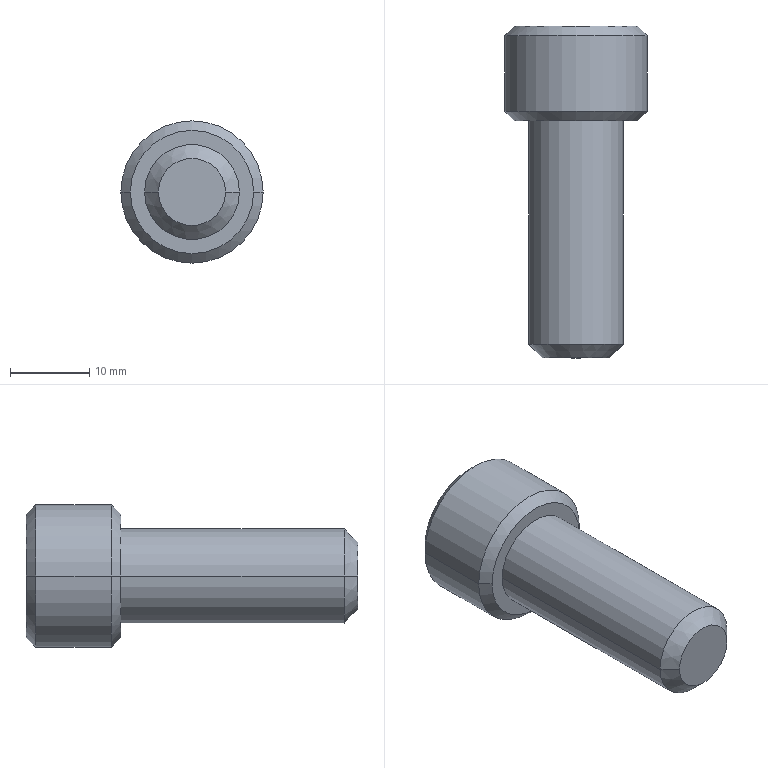Part | STEP file | BB62-M12-30L | 1 solid | 27 faces | box 18 x 42 x 18 mm | volume 5695 mm3 | plane 15 | cone 8 | cylinder 4 | commonest cylinder face diameters 12 x2 18 x2
STEP:
#1=CARTESIAN_POINT('',(0.,2.7,0.));
#2=VERTEX_POINT('',#1);
#3=CARTESIAN_POINT('',(5.715,6.,0.));
#4=VERTEX_POINT('',#3);
#5=CARTESIAN_POINT('',(0.,2.7,0.));
#6=DIRECTION('',(0.866,0.5,0.));
#7=VECTOR('',#6,1000.);
#8=LINE('',#5,#7);
#9=EDGE_CURVE('',#2,#4,#8,.T.);
#10=ORIENTED_EDGE('',*,*,#9,.F.);
#11=CARTESIAN_POINT('',(-5.715,6.,0.));
#12=VERTEX_POINT('',#11);
#13=CARTESIAN_POINT('',(0.,2.7,0.));
#14=DIRECTION('',(-0.866,0.5,0.));
#15=VECTOR('',#14,1000.);
#16=LINE('',#13,#15);
#17=EDGE_CURVE('',#2,#12,#16,.T.);
#18=ORIENTED_EDGE('',*,*,#17,.T.);
#19=CARTESIAN_POINT('',(-4.949,6.,2.857));
#20=VERTEX_POINT('',#19);
#21=CARTESIAN_POINT('',(0.,6.,0.));
#22=DIRECTION('',(0.,-1.,0.));
#23=DIRECTION('',(-1.,0.,0.));
#24=AXIS2_PLACEMENT_3D('',#21,#22,#23);
#25=CIRCLE('',#24,5.715);
#26=EDGE_CURVE('',#20,#12,#25,.T.);
#27=ORIENTED_EDGE('',*,*,#26,.F.);
#28=CARTESIAN_POINT('',(0.,6.,5.715));
#29=VERTEX_POINT('',#28);
#30=CARTESIAN_POINT('',(0.,6.,0.));
#31=DIRECTION('',(0.,-1.,0.));
#32=DIRECTION('',(-1.,0.,0.));
#33=AXIS2_PLACEMENT_3D('',#30,#31,#32);
#34=CIRCLE('',#33,5.715);
#35=EDGE_CURVE('',#29,#20,#34,.T.);
#36=ORIENTED_EDGE('',*,*,#35,.F.);
#37=CARTESIAN_POINT('',(4.949,6.,2.857));
#38=VERTEX_POINT('',#37);
#39=CARTESIAN_POINT('',(0.,6.,0.));
#40=DIRECTION('',(0.,-1.,0.));
#41=DIRECTION('',(-1.,0.,0.));
#42=AXIS2_PLACEMENT_3D('',#39,#40,#41);
#43=CIRCLE('',#42,5.715);
#44=EDGE_CURVE('',#38,#29,#43,.T.);
#45=ORIENTED_EDGE('',*,*,#44,.F.);
#46=CARTESIAN_POINT('',(0.,6.,0.));
#47=DIRECTION('',(0.,-1.,0.));
#48=DIRECTION('',(-1.,0.,0.));
#49=AXIS2_PLACEMENT_3D('',#46,#47,#48);
#50=CIRCLE('',#49,5.715);
#51=EDGE_CURVE('',#4,#38,#50,.T.);
#52=ORIENTED_EDGE('',*,*,#51,.F.);
#53=EDGE_LOOP('',(#10,#18,#27,#36,#45,#52));
#54=FACE_OUTER_BOUND('',#53,.T.);
#55=CARTESIAN_POINT('',(0.,1002.7,0.));
#56=DIRECTION('',(0.,1.,0.));
#57=DIRECTION('',(1.,0.,0.));
#58=AXIS2_PLACEMENT_3D('',#55,#56,#57);
#59=CONICAL_SURFACE('',#58,1732.051,1.047);
#60=ADVANCED_FACE('',(#54),#59,.F.);
#61=CARTESIAN_POINT('',(4.25,-30.,0.));
#62=VERTEX_POINT('',#61);
#63=CARTESIAN_POINT('',(-4.25,-30.,0.));
#64=VERTEX_POINT('',#63);
#65=CARTESIAN_POINT('',(0.,-30.,0.));
#66=DIRECTION('',(0.,1.,0.));
#67=DIRECTION('',(1.,0.,0.));
#68=AXIS2_PLACEMENT_3D('',#65,#66,#67);
#69=CIRCLE('',#68,4.25);
#70=EDGE_CURVE('',#62,#64,#69,.T.);
#71=ORIENTED_EDGE('',*,*,#70,.T.);
#72=CARTESIAN_POINT('',(-6.,-28.25,0.));
#73=VERTEX_POINT('',#72);
#74=CARTESIAN_POINT('',(-4.25,-30.,0.));
#75=DIRECTION('',(-0.7071,0.7071,0.));
#76=VECTOR('',#75,1000.);
#77=LINE('',#74,#76);
#78=EDGE_CURVE('',#64,#73,#77,.T.);
#79=ORIENTED_EDGE('',*,*,#78,.T.);
#80=CARTESIAN_POINT('',(6.,-28.25,0.));
#81=VERTEX_POINT('',#80);
#82=CARTESIAN_POINT('',(0.,-28.25,0.));
#83=DIRECTION('',(0.,-1.,0.));
#84=DIRECTION('',(-1.,0.,0.));
#85=AXIS2_PLACEMENT_3D('',#82,#83,#84);
#86=CIRCLE('',#85,6.);
#87=EDGE_CURVE('',#73,#81,#86,.T.);
#88=ORIENTED_EDGE('',*,*,#87,.T.);
#89=CARTESIAN_POINT('',(4.25,-30.,0.));
#90=DIRECTION('',(0.7071,0.7071,0.));
#91=VECTOR('',#90,1000.);
#92=LINE('',#89,#91);
#93=EDGE_CURVE('',#62,#81,#92,.T.);
#94=ORIENTED_EDGE('',*,*,#93,.F.);
#95=EDGE_LOOP('',(#71,#79,#88,#94));
#96=FACE_OUTER_BOUND('',#95,.T.);
#97=CARTESIAN_POINT('',(0.,-30.,0.));
#98=DIRECTION('',(0.,1.,0.));
#99=DIRECTION('',(1.,0.,0.));
#100=AXIS2_PLACEMENT_3D('',#97,#98,#99);
#101=CONICAL_SURFACE('',#100,4.25,0.7854);
#102=ADVANCED_FACE('',(#96),#101,.T.);
#103=ORIENTED_EDGE('',*,*,#87,.F.);
#104=CARTESIAN_POINT('',(-6.,0.,0.));
#105=VERTEX_POINT('',#104);
#106=CARTESIAN_POINT('',(-6.,-28.25,0.));
#107=DIRECTION('',(0.,1.,0.));
#108=VECTOR('',#107,1000.);
#109=LINE('',#106,#108);
#110=EDGE_CURVE('',#73,#105,#109,.T.);
#111=ORIENTED_EDGE('',*,*,#110,.T.);
#112=CARTESIAN_POINT('',(6.,0.,0.));
#113=VERTEX_POINT('',#112);
#114=CARTESIAN_POINT('',(0.,0.,0.));
#115=DIRECTION('',(0.,-1.,0.));
#116=DIRECTION('',(-1.,0.,0.));
#117=AXIS2_PLACEMENT_3D('',#114,#115,#116);
#118=CIRCLE('',#117,6.);
#119=EDGE_CURVE('',#105,#113,#118,.T.);
#120=ORIENTED_EDGE('',*,*,#119,.T.);
#121=CARTESIAN_POINT('',(6.,-28.25,0.));
#122=DIRECTION('',(0.,1.,0.));
#123=VECTOR('',#122,1000.);
#124=LINE('',#121,#123);
#125=EDGE_CURVE('',#81,#113,#124,.T.);
#126=ORIENTED_EDGE('',*,*,#125,.F.);
#127=EDGE_LOOP('',(#103,#111,#120,#126));
#128=FACE_OUTER_BOUND('',#127,.T.);
#129=CARTESIAN_POINT('',(0.,-28.25,0.));
#130=DIRECTION('',(0.,1.,0.));
#131=DIRECTION('',(1.,0.,0.));
#132=AXIS2_PLACEMENT_3D('',#129,#130,#131);
#133=CYLINDRICAL_SURFACE('',#132,6.);
#134=ADVANCED_FACE('',(#128),#133,.T.);
#135=CARTESIAN_POINT('',(-7.8,12.,0.));
#136=VERTEX_POINT('',#135);
#137=CARTESIAN_POINT('',(7.8,12.,0.));
#138=VERTEX_POINT('',#137);
#139=CARTESIAN_POINT('',(0.,12.,0.));
#140=DIRECTION('',(0.,-1.,0.));
#141=DIRECTION('',(-1.,0.,0.));
#142=AXIS2_PLACEMENT_3D('',#139,#140,#141);
#143=CIRCLE('',#142,7.8);
#144=EDGE_CURVE('',#136,#138,#143,.T.);
#145=ORIENTED_EDGE('',*,*,#144,.T.);
#146=CARTESIAN_POINT('',(9.,10.8,0.));
#147=VERTEX_POINT('',#146);
#148=CARTESIAN_POINT('',(9.,10.8,0.));
#149=DIRECTION('',(0.7071,-0.7071,0.));
#150=VECTOR('',#149,1000.);
#151=LINE('',#148,#150);
#152=EDGE_CURVE('',#138,#147,#151,.T.);
#153=ORIENTED_EDGE('',*,*,#152,.T.);
#154=CARTESIAN_POINT('',(-9.,10.8,0.));
#155=VERTEX_POINT('',#154);
#156=CARTESIAN_POINT('',(0.,10.8,0.));
#157=DIRECTION('',(0.,-1.,0.));
#158=DIRECTION('',(-1.,0.,0.));
#159=AXIS2_PLACEMENT_3D('',#156,#157,#158);
#160=CIRCLE('',#159,9.);
#161=EDGE_CURVE('',#155,#147,#160,.T.);
#162=ORIENTED_EDGE('',*,*,#161,.F.);
#163=CARTESIAN_POINT('',(-9.,10.8,0.));
#164=DIRECTION('',(-0.7071,-0.7071,0.));
#165=VECTOR('',#164,1000.);
#166=LINE('',#163,#165);
#167=EDGE_CURVE('',#136,#155,#166,.T.);
#168=ORIENTED_EDGE('',*,*,#167,.F.);
#169=EDGE_LOOP('',(#145,#153,#162,#168));
#170=FACE_OUTER_BOUND('',#169,.T.);
#171=CARTESIAN_POINT('',(0.,10.8,0.));
#172=DIRECTION('',(0.,-1.,0.));
#173=DIRECTION('',(-1.,0.,0.));
#174=AXIS2_PLACEMENT_3D('',#171,#172,#173);
#175=CONICAL_SURFACE('',#174,9.,0.7854);
#176=ADVANCED_FACE('',(#170),#175,.T.);
#177=ORIENTED_EDGE('',*,*,#161,.T.);
#178=CARTESIAN_POINT('',(9.,1.2,0.));
#179=VERTEX_POINT('',#178);
#180=CARTESIAN_POINT('',(9.,1.62,0.));
#181=DIRECTION('',(0.,-1.,0.));
#182=VECTOR('',#181,1000.);
#183=LINE('',#180,#182);
#184=EDGE_CURVE('',#147,#179,#183,.T.);
#185=ORIENTED_EDGE('',*,*,#184,.T.);
#186=CARTESIAN_POINT('',(-9.,1.2,0.));
#187=VERTEX_POINT('',#186);
#188=CARTESIAN_POINT('',(0.,1.2,0.));
#189=DIRECTION('',(0.,-1.,0.));
#190=DIRECTION('',(-1.,0.,0.));
#191=AXIS2_PLACEMENT_3D('',#188,#189,#190);
#192=CIRCLE('',#191,9.);
#193=EDGE_CURVE('',#187,#179,#192,.T.);
#194=ORIENTED_EDGE('',*,*,#193,.F.);
#195=CARTESIAN_POINT('',(-9.,1.62,0.));
#196=DIRECTION('',(0.,-1.,0.));
#197=VECTOR('',#196,1000.);
#198=LINE('',#195,#197);
#199=EDGE_CURVE('',#155,#187,#198,.T.);
#200=ORIENTED_EDGE('',*,*,#199,.F.);
#201=EDGE_LOOP('',(#177,#185,#194,#200));
#202=FACE_OUTER_BOUND('',#201,.T.);
#203=CARTESIAN_POINT('',(0.,1.62,0.));
#204=DIRECTION('',(0.,-1.,0.));
#205=DIRECTION('',(-1.,0.,0.));
#206=AXIS2_PLACEMENT_3D('',#203,#204,#205);
#207=CYLINDRICAL_SURFACE('',#206,9.);
#208=ADVANCED_FACE('',(#202),#207,.T.);
#209=CARTESIAN_POINT('',(-7.8,0.,0.));
#210=VERTEX_POINT('',#209);
#211=CARTESIAN_POINT('',(7.8,0.,0.));
#212=VERTEX_POINT('',#211);
#213=CARTESIAN_POINT('',(0.,0.,0.));
#214=DIRECTION('',(0.,-1.,0.));
#215=DIRECTION('',(-1.,0.,0.));
#216=AXIS2_PLACEMENT_3D('',#213,#214,#215);
#217=CIRCLE('',#216,7.8);
#218=EDGE_CURVE('',#210,#212,#217,.T.);
#219=ORIENTED_EDGE('',*,*,#218,.F.);
#220=CARTESIAN_POINT('',(-7.8,0.,0.));
#221=DIRECTION('',(-0.7071,0.7071,0.));
#222=VECTOR('',#221,1000.);
#223=LINE('',#220,#222);
#224=EDGE_CURVE('',#210,#187,#223,.T.);
#225=ORIENTED_EDGE('',*,*,#224,.T.);
#226=ORIENTED_EDGE('',*,*,#193,.T.);
#227=CARTESIAN_POINT('',(7.8,0.,0.));
#228=DIRECTION('',(0.7071,0.7071,0.));
#229=VECTOR('',#228,1000.);
#230=LINE('',#227,#229);
#231=EDGE_CURVE('',#212,#179,#230,.T.);
#232=ORIENTED_EDGE('',*,*,#231,.F.);
#233=EDGE_LOOP('',(#219,#225,#226,#232));
#234=FACE_OUTER_BOUND('',#233,.T.);
#235=CARTESIAN_POINT('',(0.,0.,0.));
#236=DIRECTION('',(0.,1.,0.));
#237=DIRECTION('',(1.,0.,0.));
#238=AXIS2_PLACEMENT_3D('',#235,#236,#237);
#239=CONICAL_SURFACE('',#238,7.8,0.7854);
#240=ADVANCED_FACE('',(#234),#239,.T.);
#241=ORIENTED_EDGE('',*,*,#144,.F.);
#242=CARTESIAN_POINT('',(0.,12.,0.));
#243=DIRECTION('',(0.,-1.,0.));
#244=DIRECTION('',(-1.,0.,0.));
#245=AXIS2_PLACEMENT_3D('',#242,#243,#244);
#246=CIRCLE('',#245,7.8);
#247=EDGE_CURVE('',#138,#136,#246,.T.);
#248=ORIENTED_EDGE('',*,*,#247,.F.);
#249=EDGE_LOOP('',(#241,#248));
#250=FACE_OUTER_BOUND('',#249,.T.);
#251=CARTESIAN_POINT('',(0.,12.,-5.715));
#252=VERTEX_POINT('',#251);
#253=CARTESIAN_POINT('',(-4.949,12.,-2.857));
#254=VERTEX_POINT('',#253);
#255=CARTESIAN_POINT('',(0.,12.,-5.715));
#256=DIRECTION('',(-0.866,0.,0.5));
#257=VECTOR('',#256,1000.);
#258=LINE('',#255,#257);
#259=EDGE_CURVE('',#252,#254,#258,.T.);
#260=ORIENTED_EDGE('',*,*,#259,.F.);
#261=CARTESIAN_POINT('',(4.949,12.,-2.857));
#262=VERTEX_POINT('',#261);
#263=CARTESIAN_POINT('',(4.949,12.,-2.857));
#264=DIRECTION('',(-0.866,0.,-0.5));
#265=VECTOR('',#264,1000.);
#266=LINE('',#263,#265);
#267=EDGE_CURVE('',#262,#252,#266,.T.);
#268=ORIENTED_EDGE('',*,*,#267,.F.);
#269=CARTESIAN_POINT('',(4.949,12.,2.857));
#270=VERTEX_POINT('',#269);
#271=CARTESIAN_POINT('',(4.949,12.,2.857));
#272=DIRECTION('',(0.,0.,-1.));
#273=VECTOR('',#272,1000.);
#274=LINE('',#271,#273);
#275=EDGE_CURVE('',#270,#262,#274,.T.);
#276=ORIENTED_EDGE('',*,*,#275,.F.);
#277=CARTESIAN_POINT('',(0.,12.,5.715));
#278=VERTEX_POINT('',#277);
#279=CARTESIAN_POINT('',(0.,12.,5.715));
#280=DIRECTION('',(0.866,0.,-0.5));
#281=VECTOR('',#280,1000.);
#282=LINE('',#279,#281);
#283=EDGE_CURVE('',#278,#270,#282,.T.);
#284=ORIENTED_EDGE('',*,*,#283,.F.);
#285=CARTESIAN_POINT('',(-4.949,12.,2.857));
#286=VERTEX_POINT('',#285);
#287=CARTESIAN_POINT('',(-4.949,12.,2.857));
#288=DIRECTION('',(0.866,0.,0.5));
#289=VECTOR('',#288,1000.);
#290=LINE('',#287,#289);
#291=EDGE_CURVE('',#286,#278,#290,.T.);
#292=ORIENTED_EDGE('',*,*,#291,.F.);
#293=CARTESIAN_POINT('',(-4.949,12.,-2.857));
#294=DIRECTION('',(0.,0.,1.));
#295=VECTOR('',#294,1000.);
#296=LINE('',#293,#295);
#297=EDGE_CURVE('',#254,#286,#296,.T.);
#298=ORIENTED_EDGE('',*,*,#297,.F.);
#299=EDGE_LOOP('',(#260,#268,#276,#284,#292,#298));
#300=FACE_BOUND('',#299,.T.);
#301=CARTESIAN_POINT('',(7.8,12.,0.));
#302=DIRECTION('',(0.,1.,0.));
#303=DIRECTION('',(1.,0.,0.));
#304=AXIS2_PLACEMENT_3D('',#301,#302,#303);
#305=PLANE('',#304);
#306=ADVANCED_FACE('',(#250,#300),#305,.T.);
#307=CARTESIAN_POINT('',(0.,0.,0.));
#308=DIRECTION('',(0.,-1.,0.));
#309=DIRECTION('',(-1.,0.,0.));
#310=AXIS2_PLACEMENT_3D('',#307,#308,#309);
#311=CIRCLE('',#310,6.);
#312=EDGE_CURVE('',#113,#105,#311,.T.);
#313=ORIENTED_EDGE('',*,*,#312,.F.);
#314=ORIENTED_EDGE('',*,*,#119,.F.);
#315=EDGE_LOOP('',(#313,#314));
#316=FACE_BOUND('',#315,.T.);
#317=CARTESIAN_POINT('',(0.,0.,0.));
#318=DIRECTION('',(0.,-1.,0.));
#319=DIRECTION('',(-1.,0.,0.));
#320=AXIS2_PLACEMENT_3D('',#317,#318,#319);
#321=CIRCLE('',#320,7.8);
#322=EDGE_CURVE('',#212,#210,#321,.T.);
#323=ORIENTED_EDGE('',*,*,#322,.T.);
#324=ORIENTED_EDGE('',*,*,#218,.T.);
#325=EDGE_LOOP('',(#323,#324));
#326=FACE_OUTER_BOUND('',#325,.T.);
#327=CARTESIAN_POINT('',(0.,0.,0.));
#328=DIRECTION('',(0.,-1.,0.));
#329=DIRECTION('',(-1.,0.,0.));
#330=AXIS2_PLACEMENT_3D('',#327,#328,#329);
#331=PLANE('',#330);
#332=ADVANCED_FACE('',(#316,#326),#331,.T.);
#333=ORIENTED_EDGE('',*,*,#224,.F.);
#334=ORIENTED_EDGE('',*,*,#322,.F.);
#335=ORIENTED_EDGE('',*,*,#231,.T.);
#336=CARTESIAN_POINT('',(0.,1.2,0.));
#337=DIRECTION('',(0.,-1.,0.));
#338=DIRECTION('',(-1.,0.,0.));
#339=AXIS2_PLACEMENT_3D('',#336,#337,#338);
#340=CIRCLE('',#339,9.);
#341=EDGE_CURVE('',#179,#187,#340,.T.);
#342=ORIENTED_EDGE('',*,*,#341,.T.);
#343=EDGE_LOOP('',(#333,#334,#335,#342));
#344=FACE_OUTER_BOUND('',#343,.T.);
#345=CARTESIAN_POINT('',(0.,0.,0.));
#346=DIRECTION('',(0.,1.,0.));
#347=DIRECTION('',(1.,0.,0.));
#348=AXIS2_PLACEMENT_3D('',#345,#346,#347);
#349=CONICAL_SURFACE('',#348,7.8,0.7854);
#350=ADVANCED_FACE('',(#344),#349,.T.);
#351=ORIENTED_EDGE('',*,*,#184,.F.);
#352=CARTESIAN_POINT('',(0.,10.8,0.));
#353=DIRECTION('',(0.,-1.,0.));
#354=DIRECTION('',(-1.,0.,0.));
#355=AXIS2_PLACEMENT_3D('',#352,#353,#354);
#356=CIRCLE('',#355,9.);
#357=EDGE_CURVE('',#147,#155,#356,.T.);
#358=ORIENTED_EDGE('',*,*,#357,.T.);
#359=ORIENTED_EDGE('',*,*,#199,.T.);
#360=ORIENTED_EDGE('',*,*,#341,.F.);
#361=EDGE_LOOP('',(#351,#358,#359,#360));
#362=FACE_OUTER_BOUND('',#361,.T.);
#363=CARTESIAN_POINT('',(0.,1.62,0.));
#364=DIRECTION('',(0.,-1.,0.));
#365=DIRECTION('',(-1.,0.,0.));
#366=AXIS2_PLACEMENT_3D('',#363,#364,#365);
#367=CYLINDRICAL_SURFACE('',#366,9.);
#368=ADVANCED_FACE('',(#362),#367,.T.);
#369=ORIENTED_EDGE('',*,*,#152,.F.);
#370=ORIENTED_EDGE('',*,*,#247,.T.);
#371=ORIENTED_EDGE('',*,*,#167,.T.);
#372=ORIENTED_EDGE('',*,*,#357,.F.);
#373=EDGE_LOOP('',(#369,#370,#371,#372));
#374=FACE_OUTER_BOUND('',#373,.T.);
#375=CARTESIAN_POINT('',(0.,10.8,0.));
#376=DIRECTION('',(0.,-1.,0.));
#377=DIRECTION('',(-1.,0.,0.));
#378=AXIS2_PLACEMENT_3D('',#375,#376,#377);
#379=CONICAL_SURFACE('',#378,9.,0.7854);
#380=ADVANCED_FACE('',(#374),#379,.T.);
#381=ORIENTED_EDGE('',*,*,#110,.F.);
#382=CARTESIAN_POINT('',(0.,-28.25,0.));
#383=DIRECTION('',(0.,-1.,0.));
#384=DIRECTION('',(-1.,0.,0.));
#385=AXIS2_PLACEMENT_3D('',#382,#383,#384);
#386=CIRCLE('',#385,6.);
#387=EDGE_CURVE('',#81,#73,#386,.T.);
#388=ORIENTED_EDGE('',*,*,#387,.F.);
#389=ORIENTED_EDGE('',*,*,#125,.T.);
#390=ORIENTED_EDGE('',*,*,#312,.T.);
#391=EDGE_LOOP('',(#381,#388,#389,#390));
#392=FACE_OUTER_BOUND('',#391,.T.);
#393=CARTESIAN_POINT('',(0.,-28.25,0.));
#394=DIRECTION('',(0.,1.,0.));
#395=DIRECTION('',(1.,0.,0.));
#396=AXIS2_PLACEMENT_3D('',#393,#394,#395);
#397=CYLINDRICAL_SURFACE('',#396,6.);
#398=ADVANCED_FACE('',(#392),#397,.T.);
#399=ORIENTED_EDGE('',*,*,#70,.F.);
#400=CARTESIAN_POINT('',(0.,-30.,0.));
#401=DIRECTION('',(0.,1.,0.));
#402=DIRECTION('',(1.,0.,0.));
#403=AXIS2_PLACEMENT_3D('',#400,#401,#402);
#404=CIRCLE('',#403,4.25);
#405=EDGE_CURVE('',#64,#62,#404,.T.);
#406=ORIENTED_EDGE('',*,*,#405,.F.);
#407=EDGE_LOOP('',(#399,#406));
#408=FACE_OUTER_BOUND('',#407,.T.);
#409=CARTESIAN_POINT('',(0.,-30.,0.));
#410=DIRECTION('',(0.,-1.,0.));
#411=DIRECTION('',(-1.,0.,0.));
#412=AXIS2_PLACEMENT_3D('',#409,#410,#411);
#413=PLANE('',#412);
#414=ADVANCED_FACE('',(#408),#413,.T.);
#415=ORIENTED_EDGE('',*,*,#78,.F.);
#416=ORIENTED_EDGE('',*,*,#405,.T.);
#417=ORIENTED_EDGE('',*,*,#93,.T.);
#418=ORIENTED_EDGE('',*,*,#387,.T.);
#419=EDGE_LOOP('',(#415,#416,#417,#418));
#420=FACE_OUTER_BOUND('',#419,.T.);
#421=CARTESIAN_POINT('',(0.,-30.,0.));
#422=DIRECTION('',(0.,1.,0.));
#423=DIRECTION('',(1.,0.,0.));
#424=AXIS2_PLACEMENT_3D('',#421,#422,#423);
#425=CONICAL_SURFACE('',#424,4.25,0.7854);
#426=ADVANCED_FACE('',(#420),#425,.T.);
#427=CARTESIAN_POINT('',(4.949,6.,-2.858));
#428=VERTEX_POINT('',#427);
#429=CARTESIAN_POINT('',(0.,6.,-5.715));
#430=VERTEX_POINT('',#429);
#431=CARTESIAN_POINT('',(4.949,6.,-2.857));
#432=DIRECTION('',(-0.866,0.,-0.5));
#433=VECTOR('',#432,1000.);
#434=LINE('',#431,#433);
#435=EDGE_CURVE('',#428,#430,#434,.T.);
#436=ORIENTED_EDGE('',*,*,#435,.F.);
#437=CARTESIAN_POINT('',(4.949,12.,-2.857));
#438=DIRECTION('',(0.,-1.,0.));
#439=VECTOR('',#438,1000.);
#440=LINE('',#437,#439);
#441=EDGE_CURVE('',#262,#428,#440,.T.);
#442=ORIENTED_EDGE('',*,*,#441,.F.);
#443=ORIENTED_EDGE('',*,*,#267,.T.);
#444=CARTESIAN_POINT('',(0.,12.,-5.715));
#445=DIRECTION('',(0.,-1.,0.));
#446=VECTOR('',#445,1000.);
#447=LINE('',#444,#446);
#448=EDGE_CURVE('',#252,#430,#447,.T.);
#449=ORIENTED_EDGE('',*,*,#448,.T.);
#450=EDGE_LOOP('',(#436,#442,#443,#449));
#451=FACE_OUTER_BOUND('',#450,.T.);
#452=CARTESIAN_POINT('',(4.949,12.,-2.857));
#453=DIRECTION('',(-0.5,0.,0.866));
#454=DIRECTION('',(0.866,0.,0.5));
#455=AXIS2_PLACEMENT_3D('',#452,#453,#454);
#456=PLANE('',#455);
#457=ADVANCED_FACE('',(#451),#456,.T.);
#458=CARTESIAN_POINT('',(-4.949,6.,-2.857));
#459=VERTEX_POINT('',#458);
#460=CARTESIAN_POINT('',(0.,6.,-5.715));
#461=DIRECTION('',(-0.866,0.,0.5));
#462=VECTOR('',#461,1000.);
#463=LINE('',#460,#462);
#464=EDGE_CURVE('',#430,#459,#463,.T.);
#465=ORIENTED_EDGE('',*,*,#464,.F.);
#466=ORIENTED_EDGE('',*,*,#448,.F.);
#467=ORIENTED_EDGE('',*,*,#259,.T.);
#468=CARTESIAN_POINT('',(-4.949,12.,-2.857));
#469=DIRECTION('',(0.,-1.,0.));
#470=VECTOR('',#469,1000.);
#471=LINE('',#468,#470);
#472=EDGE_CURVE('',#254,#459,#471,.T.);
#473=ORIENTED_EDGE('',*,*,#472,.T.);
#474=EDGE_LOOP('',(#465,#466,#467,#473));
#475=FACE_OUTER_BOUND('',#474,.T.);
#476=CARTESIAN_POINT('',(0.,12.,-5.715));
#477=DIRECTION('',(0.5,0.,0.866));
#478=DIRECTION('',(0.866,0.,-0.5));
#479=AXIS2_PLACEMENT_3D('',#476,#477,#478);
#480=PLANE('',#479);
#481=ADVANCED_FACE('',(#475),#480,.T.);
#482=CARTESIAN_POINT('',(-4.949,6.,-2.857));
#483=DIRECTION('',(0.,0.,1.));
#484=VECTOR('',#483,1000.);
#485=LINE('',#482,#484);
#486=EDGE_CURVE('',#459,#20,#485,.T.);
#487=ORIENTED_EDGE('',*,*,#486,.F.);
#488=ORIENTED_EDGE('',*,*,#472,.F.);
#489=ORIENTED_EDGE('',*,*,#297,.T.);
#490=CARTESIAN_POINT('',(-4.949,12.,2.857));
#491=DIRECTION('',(0.,-1.,0.));
#492=VECTOR('',#491,1000.);
#493=LINE('',#490,#492);
#494=EDGE_CURVE('',#286,#20,#493,.T.);
#495=ORIENTED_EDGE('',*,*,#494,.T.);
#496=EDGE_LOOP('',(#487,#488,#489,#495));
#497=FACE_OUTER_BOUND('',#496,.T.);
#498=CARTESIAN_POINT('',(-4.949,12.,-2.857));
#499=DIRECTION('',(1.,0.,0.));
#500=DIRECTION('',(0.,0.,-1.));
#501=AXIS2_PLACEMENT_3D('',#498,#499,#500);
#502=PLANE('',#501);
#503=ADVANCED_FACE('',(#497),#502,.T.);
#504=CARTESIAN_POINT('',(-4.949,6.,2.857));
#505=DIRECTION('',(0.866,0.,0.5));
#506=VECTOR('',#505,1000.);
#507=LINE('',#504,#506);
#508=EDGE_CURVE('',#20,#29,#507,.T.);
#509=ORIENTED_EDGE('',*,*,#508,.F.);
#510=ORIENTED_EDGE('',*,*,#494,.F.);
#511=ORIENTED_EDGE('',*,*,#291,.T.);
#512=CARTESIAN_POINT('',(0.,12.,5.715));
#513=DIRECTION('',(0.,-1.,0.));
#514=VECTOR('',#513,1000.);
#515=LINE('',#512,#514);
#516=EDGE_CURVE('',#278,#29,#515,.T.);
#517=ORIENTED_EDGE('',*,*,#516,.T.);
#518=EDGE_LOOP('',(#509,#510,#511,#517));
#519=FACE_OUTER_BOUND('',#518,.T.);
#520=CARTESIAN_POINT('',(-4.949,12.,2.857));
#521=DIRECTION('',(0.5,0.,-0.866));
#522=DIRECTION('',(-0.866,0.,-0.5));
#523=AXIS2_PLACEMENT_3D('',#520,#521,#522);
#524=PLANE('',#523);
#525=ADVANCED_FACE('',(#519),#524,.T.);
#526=CARTESIAN_POINT('',(0.,6.,5.715));
#527=DIRECTION('',(0.866,0.,-0.5));
#528=VECTOR('',#527,1000.);
#529=LINE('',#526,#528);
#530=EDGE_CURVE('',#29,#38,#529,.T.);
#531=ORIENTED_EDGE('',*,*,#530,.F.);
#532=ORIENTED_EDGE('',*,*,#516,.F.);
#533=ORIENTED_EDGE('',*,*,#283,.T.);
#534=CARTESIAN_POINT('',(4.949,12.,2.857));
#535=DIRECTION('',(0.,-1.,0.));
#536=VECTOR('',#535,1000.);
#537=LINE('',#534,#536);
#538=EDGE_CURVE('',#270,#38,#537,.T.);
#539=ORIENTED_EDGE('',*,*,#538,.T.);
#540=EDGE_LOOP('',(#531,#532,#533,#539));
#541=FACE_OUTER_BOUND('',#540,.T.);
#542=CARTESIAN_POINT('',(0.,12.,5.715));
#543=DIRECTION('',(-0.5,0.,-0.866));
#544=DIRECTION('',(-0.866,0.,0.5));
#545=AXIS2_PLACEMENT_3D('',#542,#543,#544);
#546=PLANE('',#545);
#547=ADVANCED_FACE('',(#541),#546,.T.);
#548=CARTESIAN_POINT('',(4.949,6.,2.857));
#549=DIRECTION('',(0.,0.,-1.));
#550=VECTOR('',#549,1000.);
#551=LINE('',#548,#550);
#552=EDGE_CURVE('',#38,#428,#551,.T.);
#553=ORIENTED_EDGE('',*,*,#552,.F.);
#554=ORIENTED_EDGE('',*,*,#538,.F.);
#555=ORIENTED_EDGE('',*,*,#275,.T.);
#556=ORIENTED_EDGE('',*,*,#441,.T.);
#557=EDGE_LOOP('',(#553,#554,#555,#556));
#558=FACE_OUTER_BOUND('',#557,.T.);
#559=CARTESIAN_POINT('',(4.949,12.,2.857));
#560=DIRECTION('',(-1.,0.,0.));
#561=DIRECTION('',(0.,0.,1.));
#562=AXIS2_PLACEMENT_3D('',#559,#560,#561);
#563=PLANE('',#562);
#564=ADVANCED_FACE('',(#558),#563,.T.);
#565=ORIENTED_EDGE('',*,*,#435,.T.);
#566=CARTESIAN_POINT('',(0.,6.,0.));
#567=DIRECTION('',(0.,-1.,0.));
#568=DIRECTION('',(-1.,0.,0.));
#569=AXIS2_PLACEMENT_3D('',#566,#567,#568);
#570=CIRCLE('',#569,5.715);
#571=EDGE_CURVE('',#430,#428,#570,.T.);
#572=ORIENTED_EDGE('',*,*,#571,.T.);
#573=EDGE_LOOP('',(#565,#572));
#574=FACE_OUTER_BOUND('',#573,.T.);
#575=CARTESIAN_POINT('',(0.,6.,0.));
#576=DIRECTION('',(0.,1.,0.));
#577=DIRECTION('',(1.,0.,0.));
#578=AXIS2_PLACEMENT_3D('',#575,#576,#577);
#579=PLANE('',#578);
#580=ADVANCED_FACE('',(#574),#579,.F.);
#581=ORIENTED_EDGE('',*,*,#552,.T.);
#582=CARTESIAN_POINT('',(0.,6.,0.));
#583=DIRECTION('',(0.,-1.,0.));
#584=DIRECTION('',(-1.,0.,0.));
#585=AXIS2_PLACEMENT_3D('',#582,#583,#584);
#586=CIRCLE('',#585,5.715);
#587=EDGE_CURVE('',#428,#4,#586,.T.);
#588=ORIENTED_EDGE('',*,*,#587,.T.);
#589=ORIENTED_EDGE('',*,*,#51,.T.);
#590=EDGE_LOOP('',(#581,#588,#589));
#591=FACE_OUTER_BOUND('',#590,.T.);
#592=CARTESIAN_POINT('',(0.,6.,0.));
#593=DIRECTION('',(0.,1.,0.));
#594=DIRECTION('',(1.,0.,0.));
#595=AXIS2_PLACEMENT_3D('',#592,#593,#594);
#596=PLANE('',#595);
#597=ADVANCED_FACE('',(#591),#596,.F.);
#598=ORIENTED_EDGE('',*,*,#530,.T.);
#599=ORIENTED_EDGE('',*,*,#44,.T.);
#600=EDGE_LOOP('',(#598,#599));
#601=FACE_OUTER_BOUND('',#600,.T.);
#602=CARTESIAN_POINT('',(0.,6.,0.));
#603=DIRECTION('',(0.,1.,0.));
#604=DIRECTION('',(1.,0.,0.));
#605=AXIS2_PLACEMENT_3D('',#602,#603,#604);
#606=PLANE('',#605);
#607=ADVANCED_FACE('',(#601),#606,.F.);
#608=ORIENTED_EDGE('',*,*,#508,.T.);
#609=ORIENTED_EDGE('',*,*,#35,.T.);
#610=EDGE_LOOP('',(#608,#609));
#611=FACE_OUTER_BOUND('',#610,.T.);
#612=CARTESIAN_POINT('',(0.,6.,0.));
#613=DIRECTION('',(0.,1.,0.));
#614=DIRECTION('',(1.,0.,0.));
#615=AXIS2_PLACEMENT_3D('',#612,#613,#614);
#616=PLANE('',#615);
#617=ADVANCED_FACE('',(#611),#616,.F.);
#618=ORIENTED_EDGE('',*,*,#486,.T.);
#619=ORIENTED_EDGE('',*,*,#26,.T.);
#620=CARTESIAN_POINT('',(0.,6.,0.));
#621=DIRECTION('',(0.,-1.,0.));
#622=DIRECTION('',(-1.,0.,0.));
#623=AXIS2_PLACEMENT_3D('',#620,#621,#622);
#624=CIRCLE('',#623,5.715);
#625=EDGE_CURVE('',#12,#459,#624,.T.);
#626=ORIENTED_EDGE('',*,*,#625,.T.);
#627=EDGE_LOOP('',(#618,#619,#626));
#628=FACE_OUTER_BOUND('',#627,.T.);
#629=CARTESIAN_POINT('',(0.,6.,0.));
#630=DIRECTION('',(0.,1.,0.));
#631=DIRECTION('',(1.,0.,0.));
#632=AXIS2_PLACEMENT_3D('',#629,#630,#631);
#633=PLANE('',#632);
#634=ADVANCED_FACE('',(#628),#633,.F.);
#635=ORIENTED_EDGE('',*,*,#464,.T.);
#636=CARTESIAN_POINT('',(0.,6.,0.));
#637=DIRECTION('',(0.,-1.,0.));
#638=DIRECTION('',(-1.,0.,0.));
#639=AXIS2_PLACEMENT_3D('',#636,#637,#638);
#640=CIRCLE('',#639,5.715);
#641=EDGE_CURVE('',#459,#430,#640,.T.);
#642=ORIENTED_EDGE('',*,*,#641,.T.);
#643=EDGE_LOOP('',(#635,#642));
#644=FACE_OUTER_BOUND('',#643,.T.);
#645=CARTESIAN_POINT('',(0.,6.,0.));
#646=DIRECTION('',(0.,1.,0.));
#647=DIRECTION('',(1.,0.,0.));
#648=AXIS2_PLACEMENT_3D('',#645,#646,#647);
#649=PLANE('',#648);
#650=ADVANCED_FACE('',(#644),#649,.F.);
#651=ORIENTED_EDGE('',*,*,#17,.F.);
#652=ORIENTED_EDGE('',*,*,#9,.T.);
#653=ORIENTED_EDGE('',*,*,#587,.F.);
#654=ORIENTED_EDGE('',*,*,#571,.F.);
#655=ORIENTED_EDGE('',*,*,#641,.F.);
#656=ORIENTED_EDGE('',*,*,#625,.F.);
#657=EDGE_LOOP('',(#651,#652,#653,#654,#655,#656));
#658=FACE_OUTER_BOUND('',#657,.T.);
#659=CARTESIAN_POINT('',(0.,1002.7,0.));
#660=DIRECTION('',(0.,1.,0.));
#661=DIRECTION('',(1.,0.,0.));
#662=AXIS2_PLACEMENT_3D('',#659,#660,#661);
#663=CONICAL_SURFACE('',#662,1732.051,1.047);
#664=ADVANCED_FACE('',(#658),#663,.F.);
#665=CLOSED_SHELL('',(#60,#102,#134,#176,#208,#240,#306,#332,#350,#368,#380,#398,#414,#426,#457,#481,#503,#525,#547,#564,#580,#597,#607,#617,#634,#650,#664));
#666=MANIFOLD_SOLID_BREP('',#665);
#667=CARTESIAN_POINT('',(0.,0.,0.));
#668=DIRECTION('',(0.,0.,1.));
#669=DIRECTION('',(1.,0.,0.));
#670=AXIS2_PLACEMENT_3D('',#667,#668,#669);
#671=(LENGTH_UNIT()NAMED_UNIT(*)SI_UNIT(.MILLI.,.METRE.));
#672=UNCERTAINTY_MEASURE_WITH_UNIT(LENGTH_MEASURE(0.00001),#671,'','');
#673=(NAMED_UNIT(*)PLANE_ANGLE_UNIT()SI_UNIT($,.RADIAN.));
#674=(NAMED_UNIT(*)SI_UNIT($,.STERADIAN.)SOLID_ANGLE_UNIT());
#675=(GEOMETRIC_REPRESENTATION_CONTEXT(3)GLOBAL_UNCERTAINTY_ASSIGNED_CONTEXT((#672))GLOBAL_UNIT_ASSIGNED_CONTEXT((#671,#673,#674))REPRESENTATION_CONTEXT('',''));
#676=ADVANCED_BREP_SHAPE_REPRESENTATION('',(#666,#670),#675);